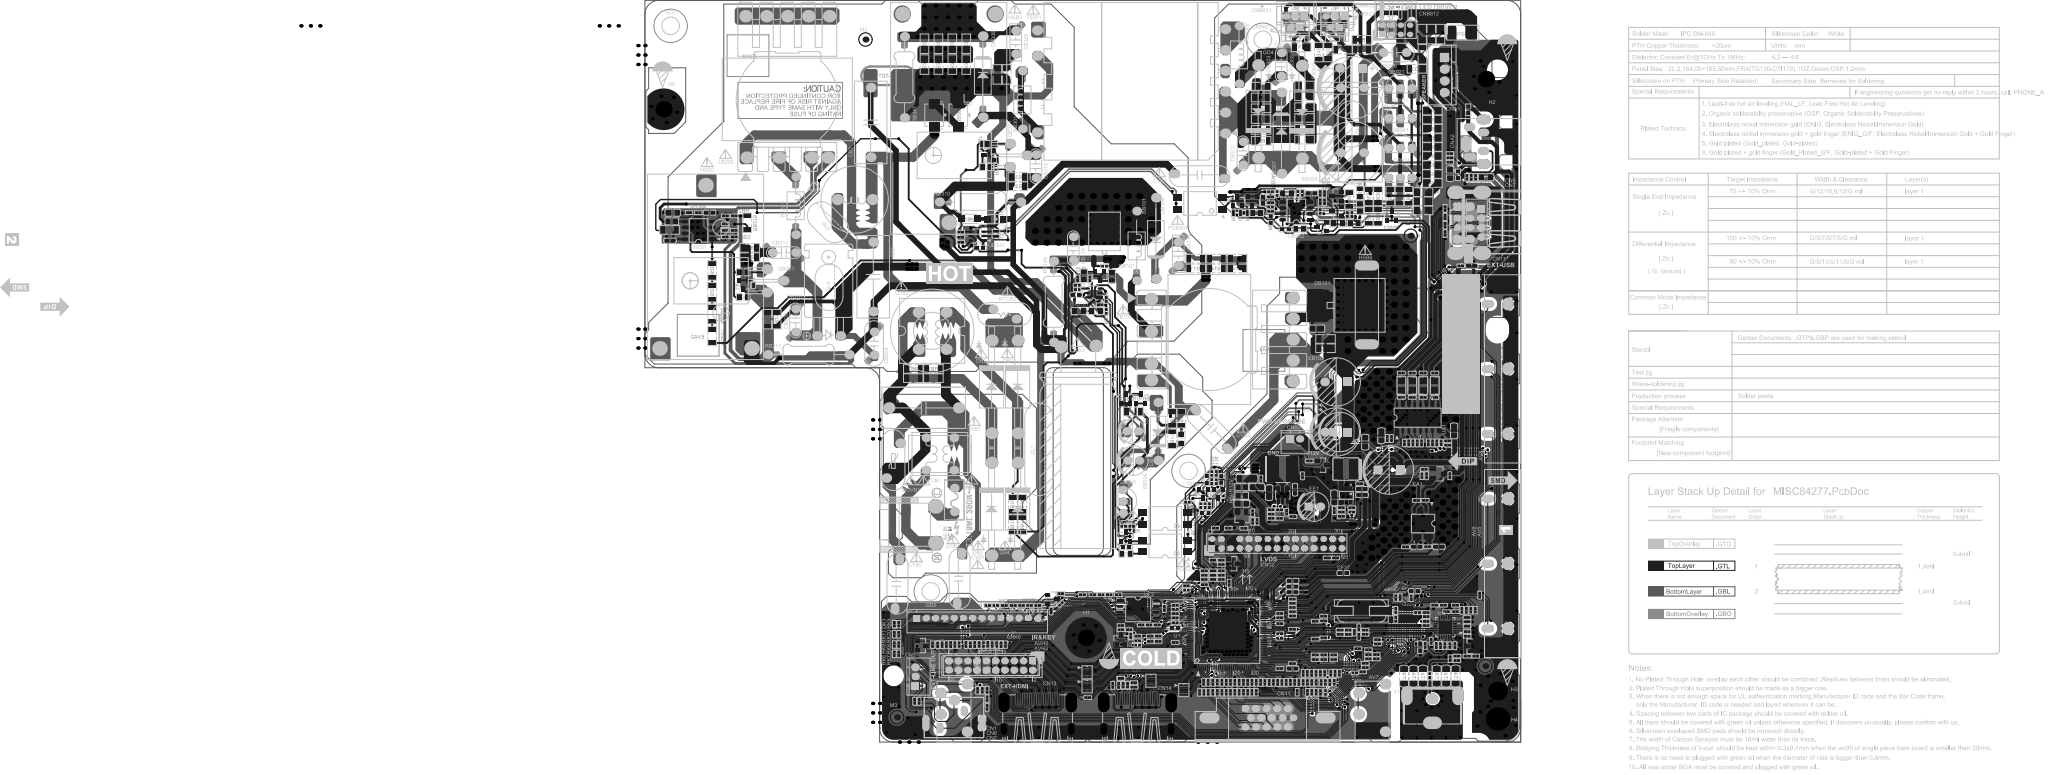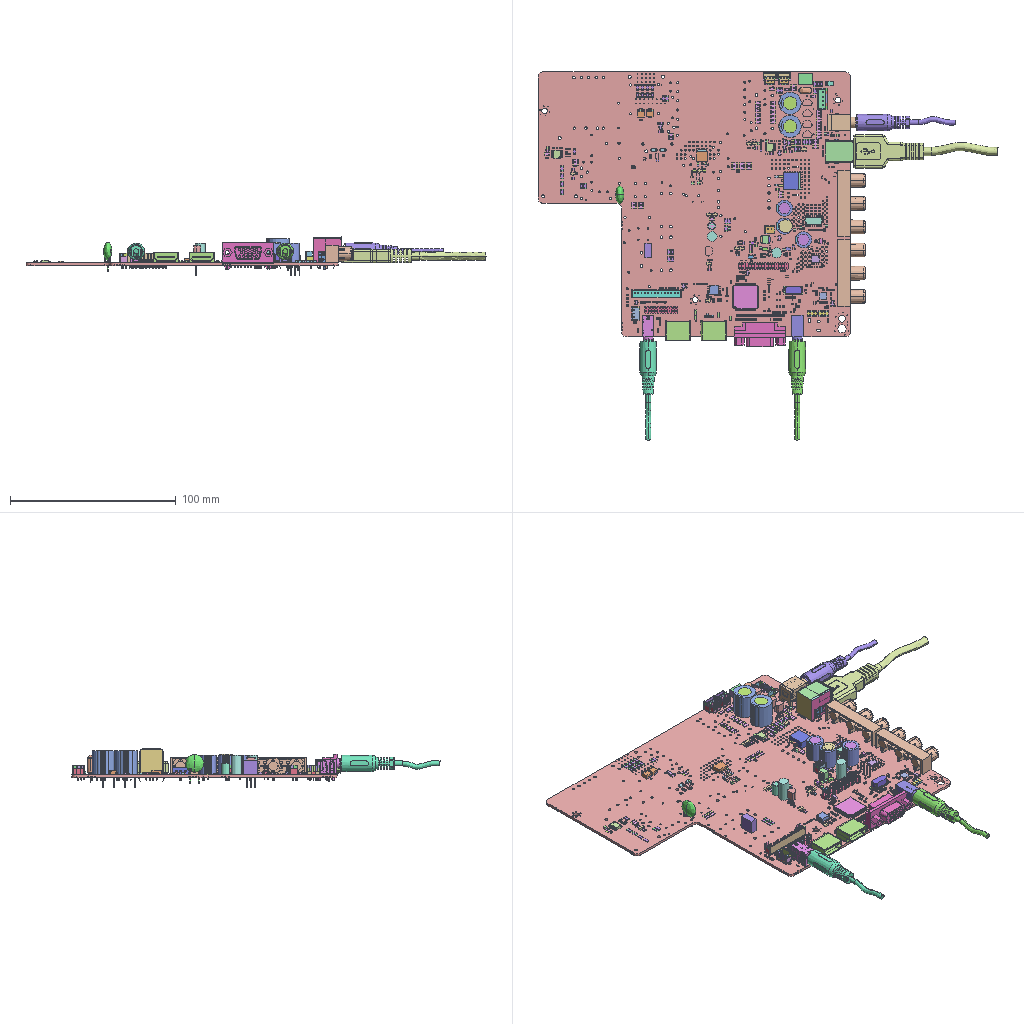Circuit board layout | Altium Designer | box 277.7 x 222.2 x 23.8 mm
Layer stack:
# Altium Designer layer stack of  (unit mm; dielectric type: 0 none, 1 core, 2 prepreg, 3 surface material)
index,name,kind,layer,copper_thickness_mm,dielectric_type,dielectric_thickness_mm,dielectric_material,dielectric_constant
0,TopPaste,other,,,,,,
1,TopOverlay,other,,,,,,
2,TopSolder,dielectric,,,3,0.0102,Solder Resist,3.5
3,TopLayer,copper,TopLayer,0.0356,,,,
4,Dielectric1,dielectric,,,1,1.5,FR-4,4.8
5,BottomLayer,copper,BottomLayer,0.0356,,,,
6,BottomSolder,dielectric,,,3,0.0102,Solder Resist,3.5
7,BottomOverlay,other,,,,,,
8,BottomPaste,other,,,,,,
# drill layer pairs: low layer,high layer
drill_pair,TopLayer,BottomLayer
Part placement, first 448 of 710 lines:
Designator,Comment,Layer,Footprint,Center-X(mm),Center-Y(mm),Rotation
NO DOLBY,NO DOLBY,BottomLayer,NO_DOLBY-SILK,-669.474,-465.296,360
CNB1,Connect jack, 2Pin, D7.92, L, SNAP, Fool-proofing, nature, L=2.8mm, DIP, AMA,TopLayer,CON2-H7.92,-126,46.889,360
S/N1,Barcode,TopLayer,Barcode,-669.474,-465.296,90
EVA6,NC/7×7×3mm-C-4305 fireproof foam-black,BottomLayer,EVA(7*7*3),-669.474,-465.296,180
S/N2,Barcode,BottomLayer,BARCODE,-669.474,-465.296,0
UF2,SPI FLASH chip, IC SPI FLASH, 32Mb, SOIC8, SMD, GD25Q32CSIG, GigaDevice,TopLayer,SOIC8,-82.347,28.626,360
RH20,NC/NC/100ohm-0402-±5%-1/16W,TopLayer,R0402,-86.063,24.232,180
RH19,NC/NC/100ohm-0402-±5%-1/16W,TopLayer,R0402,-86.063,25.138,180
AVH3,NC/gold pin, pin connector, 2×10Pin, D, D2.0mm, L=2.6mm, DIP, LK,TopLayer,SIP2*10/2.0DM-1,-114.1,16.518,360
AVH2,NC/NC/connect jack, 2×10Pin, D2.0, D, SNAP, Fool-proofing, Beige, L=2.6mm, DIP, CJ,TopLayer,SIP2*10/2.0D-4,-114.1,16.518,360
RT7,FCM1005KF-121T06(120ohm-500mA),TopLayer,R0402,-23.581,31.1,270
RT12,430ohm-0402-±5%-1/16W,TopLayer,R0402,-35.8,23.7,90
LF7,0ohm-0402-±5%-1/16W,TopLayer,L0402,-20.371,27.058,0
CT2,NC/10uF-0603-X5R-±20%-6.3V,TopLayer,C0603,-22.835,32.558,360
CF39,NC/4.7pF-0402-NPO-±5%-50V,TopLayer,C0402,-20.371,27.94,180
CF33,1000pF-0402-X7R-±10%-50V,TopLayer,C0402,-22.2,27.94,180
CF32,1Kohm-0402-±5%-1/16W,TopLayer,C0402,-26.9,28.407,90
UB102,AZ431AN-ATRE1(BCD),TopLayer,SOT-23-RAK,-65.15,53.575,180
RB135,18Kohm-0402-±1%-1/16W,TopLayer,R0402,-65.55,56.15,90
RB134,4K7ohm-0402-±1%-1/16W,TopLayer,R0402,-65.55,57.95,90
RB133,3Kohm-0402-±1%-1/16W,TopLayer,R0402,-66.5,57.95,270
RB132,3Kohm-0402-±1%-1/16W,TopLayer,R0402,-71.75,51.75,180
RB131,2Kohm-0603-±5%-1/10W,TopLayer,R0603,-64.45,56.65,90
CB110,NC/1000pF-0402-X7R-±10%-50V,TopLayer,C0402,-66.5,56.15,90
CB109,0.1uF-0603-X7R-±10%-50V,TopLayer,C0603,-67.6,56.65,90
RB386,9K1ohm-0402-±1%-1/16W,TopLayer,R0402,-68.879,50.952,270
RB385,4K7ohm-0402-±1%-1/16W,TopLayer,R0402,-67.952,50.952,90
RB384,1Kohm-0603-±1%-1/10W,TopLayer,R0603,-67.952,49.4,180
QB305,LMBT3904LT1G,TopLayer,SOT-23,-68.35,53.575,360
CB327,0.1uF-0402-X7R-±10%-16V,TopLayer,C0402,-67.029,50.952,270
RB146,100Kohm-1206-±5%-1/4W,TopLayer,R1206,-65.515,102.159,360
RB145,100Kohm-1206-±5%-1/4W,TopLayer,R1206,-61.068,104.286,360
RB144,100Kohm-1206-±5%-1/4W,TopLayer,R1206,-65.515,104.286,360
HSB2,40×25×5.0-black-with pins (thickness=1.5mm)-FR,TopLayer,HS018,-175.489,102.514,0
DB105,FR107 (tape and reel/LRC),TopLayer,D1-H-12.5,-78.08,67.018,270
DB202,NC/GS3J-B(GULF),TopLayer,DIODE-SMB-1,-126.287,135.215,270
DB370,NC/FF7,TopLayer,DIODE-S-14,-118.624,112.856,180
DB371,NC/FF7,TopLayer,DIODE-S-14,-113.05,112.827,180
GL3,NC/SLD-8854W,TopLayer,Silica_gel-10,-669.474,-465.296,45
RB347,NC/MOF-300Kohm-±5%-2WS (tape and reel/Futaba),TopLayer,R2-H-17.5,-132.664,143.421,270
LF5,NC,TopLayer,GND,-73.937,26.294,270
LF3,NC,TopLayer,GND,-49.345,22.913,360
LF2,NC,TopLayer,GND,-52.903,16.325,135
LF1,NC,TopLayer,GND,-49.373,23.531,360
C1,NC/10uF-1206-X5R-±10%-16V,TopLayer,C1206,-58.95,56.85,360
H5,Location hole,TopLayer,ASSE3.5C-3,-184.446,136.466,0
M3,MARK,TopLayer,MARK,-134.254,5.359,0
M2,MARK,TopLayer,MARK,-141.05,151.55,0
COLD,COLD,TopLayer,COLD,-669.474,-465.296,360
CAUTION,CAUTION,BottomLayer,CAUTION,-669.474,-465.296,180
T1,RF connector,RF JACK,H,IEC,T14.5,CH6.3,12.4×13.2×7.7mm,DIP,LHD-020 assembly,LHD,TopLayer,ANT-IEC14.5-H-短体-NG,-19,7.079,360
CD5,10uF-0805-X5R-±20%-16V,TopLayer,C0805,-54.171,53.831,270
5V_STB,TEST,BottomLayer,TP,-33.96,47.024,90
CM2,0.1uF-0402-X5R-±20%-16V,TopLayer,C0402,-15.265,57.455,270
QM1,WPM2341A-3/TR,TopLayer,SOT-23-1,-17.78,57.861,90
??,NC/glue, 0.1g, silicone,TopLayer,HEAT-SHRINKABLE_TUBE,-1.778,1.778,90
CN17,NC/4PIN-2.0-D-H-G,TopLayer,SIP4/2.0D-1,-8.521,111.989,270
RA14,NC/120ohm-0402-±5%-1/16W,TopLayer,R0402,-15.246,126.944,360
RA17,NC/0ohm-0603-±5%-1/10W,TopLayer,R0603,-11.3,136.4,90
RA9,NC/120ohm-0402-±5%-1/16W,TopLayer,R0402,-11.59,121.831,90
CA41,10uF-0805-X5R-±20%-16V,TopLayer,C0805,-15.197,122.616,270
CA40,10uF-0805-X5R-±20%-16V,TopLayer,C0805,-7.475,121.831,360
CA61,6800pF-0402-X7R-±10%-50V,TopLayer,C0402,-15.246,126.022,180
CA60,6800pF-0402-X7R-±10%-50V,TopLayer,C0402,-10.663,121.831,270
RA10,NC/0ohm-0603-±5%-1/10W,TopLayer,R0603,-13.503,122.372,90
RA23,1Kohm-0402-±5%-1/16W,TopLayer,R0402,-9.723,121.831,270
RA28,1Kohm-0402-±5%-1/16W,TopLayer,R0402,-15.246,125.092,180
U1,TV main chip,IC Main Chip,TSUMV56RUU-Z1,32bit,Single-Core,QFP,SMD,Mstar,TopLayer,QFP128/0.4-5,-63.232,24.046,0
M1,MARK,TopLayer,MARK,-7.62,16.383,0
H4,Location hole,TopLayer,ASSE5.0C-4,-5.267,5.093,0
H3,Location hole,TopLayer,ASSE4.0C-4,-5.216,11.22,0
H2,Location hole,TopLayer,ASSE3.5C-3,-7.436,143.528,0
H1,Location hole,TopLayer,ASSE3.5C-3,-93.537,22.466,0
CNA2,PJ-339,TopLayer,PHONE-HD-12,-7.45,129.5,90
CNA1,Connect jack, 4Pin, D2.50, D, L=2.8mm, DIP, LD,TopLayer,SIP4/2.54D-1,-16.421,143.887,270
CN14,161011041,TopLayer,HDMI-HS-1,-82.5,5.92,0
CN13,161011041,TopLayer,HDMI-HS-1,-104,5.92,0
CN11,WLHD-051A,TopLayer,DB15-HF-1,-54.5,5.251,0
CN7,NC/USB-042M-002DP,TopLayer,USB1-HD-2,-9.655,112,90
CN6,NC/earphone terminal, Earphone Jack, H, F3.5, CH7.0, Black, switch, Seal, DIP, PJ7724-F05L3BY-D, YUQIU,TopLayer,PHONE-HD-42,-122.1,7.371,0
CN5,WLUS-074B,TopLayer,USB2-HD-1,-11.15,112,90
CN2,NC/RCA terminal, RCA Jack, AV1, H, Orange, CH5.5, Seal, DIP, AV38A-01S-5020, QS,TopLayer,AV1-H-4,-122.002,6.546,0
CN1,RCA terminal, RCA Jack, AV1, H, Yellow, CH5.5, Seal, DIP, AV38A-01S-5030, QS,TopLayer,AV1-H-4,-122.002,6.546,0
AV8,RCA terminal, RCA Jack, AV3, H, Yellow, White, Red, CH5.5, D14, Seal, DIP, RC075-F03L3BY-A, YUQIU (MI material),TopLayer,AV3-H14-15,-4.925,80.5,90
AV7,Earphone terminal, Earphone Jack, H, F3.5, CH7.0, Black, Seal, DIP, PJ7723-F03L3BY-C, YUQIU,TopLayer,PHONE-HD-41,-32.05,7.375,0
AV5,NC/RCA terminal, RCA Jack, AV3, H, Green, Blue, Red, CH5.5, D14, Seal, DIP, RC075-F03L3BY-B, YUQIU (MI material),TopLayer,AV3-H14-15,-4.925,38.5,90
AV2,RCA terminal, RCA Jack, AV3, H, Yellow, White, Red, CH5.5, D14, Seal, DIP, RC075-F03L3BY-A, YUQIU (MI material),TopLayer,AV3-H14-15,-4.925,38.5,90
CQC,CQC,TopLayer,CQC,-669.474,-465.296,270
Manufacture_Info,Manufacture_Info,TopLayer,MANUFACTURE_INFO,-36.802,95.208,360
XXXXXXXXXXXX,PCB_NAME,TopLayer,PCB_NAME,-39.624,32.334,90
CA23,0.1uF-0402-X5R-±20%-16V,TopLayer,C0402,-28.727,65.481,90
RA8,4K7ohm-0402-±5%-1/16W,TopLayer,R0402,-64.44,38.303,180
CA22,0.22uF-0402-X5R-±10%-16V,TopLayer,C0402,-18.491,74.346,180
CA13,0.22uF-0402-X5R-±10%-16V,TopLayer,C0402,-21.006,74.346,360
CA12,0.22uF-0402-X5R-±10%-16V,TopLayer,C0402,-23.368,74.346,180
CA20,0.22uF-0402-X5R-±10%-16V,TopLayer,C0402,-18.986,64.529,270
CA21,0.22uF-0402-X5R-±10%-16V,TopLayer,C0402,-19.907,64.529,270
CA15,1uF-0402-X5R-±20%-16V,TopLayer,C0402,-21.361,64.529,90
RA1,4K7ohm-0402-±5%-1/16W,TopLayer,R0402,-64.44,36.932,360
CA9,1000pF-0402-X7R-±10%-50V,TopLayer,C0402,-15.723,64.058,180
CA10,2200pF-0402-X7R-±10%-50V,TopLayer,C0402,-18.491,79.604,360
CA11,0.1uF-0402-X5R-±20%-16V,TopLayer,C0402,-15.723,64.973,180
CA14,0.22uF-0402-X5R-±10%-16V,TopLayer,C0402,-25.705,74.346,360
CA17,2200pF-0402-X7R-±10%-50V,TopLayer,C0402,-21.006,79.604,180
LBA1,UPZ2012E601-2R0TF(600ohm-2000mA),TopLayer,L0805,-25.705,76.911,90
LBA2,UPZ2012E601-2R0TF(600ohm-2000mA),TopLayer,L0805,-23.368,76.911,90
LBA3,UPZ2012E601-2R0TF(600ohm-2000mA),TopLayer,L0805,-21.006,76.911,90
LBA4,UPZ2012E601-2R0TF(600ohm-2000mA),TopLayer,L0805,-18.491,76.911,90
CT46,NC/4700pF-1206-X7R-±10%-1000V,TopLayer,C1206,-14.026,14.243,270
CT43,0ohm-1206-±5%-1/4W,TopLayer,C1206,-18.09,14.243,270
CT42,0ohm-1206-±5%-1/4W,TopLayer,C1206,-16.058,14.243,270
CT41,0ohm-1206-±5%-1/4W,TopLayer,C1206,-21.049,14.218,270
CT44,0ohm-1206-±5%-1/4W,TopLayer,C1206,-23.081,14.218,270
CT40,470pF-0402-X7R-±10%-50V,TopLayer,C0402,-19.563,14.307,90
CT45,NC/4700pF-1206-X7R-±10%-1000V,TopLayer,C1206,-25.113,14.218,270
RT4,4K7ohm-0402-±5%-1/16W,TopLayer,R0402,-25.951,31.168,270
RT3,4K7ohm-0402-±5%-1/16W,TopLayer,R0402,-26.9,31.168,270
CT30,0.1uF-0402-X5R-±20%-16V,TopLayer,C0402,-18.517,29.54,360
CT9,0.1uF-0402-X5R-±20%-16V,TopLayer,C0402,-14.161,20.813,270
CT11,0.022uF-0402-X7R-±10%-16V,TopLayer,C0402,-17.271,20.837,90
CT12,0.022uF-0402-X7R-±10%-16V,TopLayer,C0402,-18.186,20.837,270
CT18,0.1uF-0402-X5R-±20%-16V,TopLayer,C0402,-19.281,21.742,90
CT21,0.047uF-0402-X7R-±10%-16V,TopLayer,C0402,-11.573,25.969,360
CT25,0.1uF-0402-X5R-±20%-16V,TopLayer,C0402,-12.673,28.414,90
CT26,330pF-0402-NPO-±5%-50V,TopLayer,C0402,-16,28.135,360
CT27,0.1uF-0402-X5R-±20%-16V,TopLayer,C0402,-16.647,29.527,360
CT29,6800pF-0402-X7R-±10%-50V,TopLayer,C0402,-14.044,29.527,360
DT1,BAV99-BR,TopLayer,SO-23,-10.671,20.686,270
LT1,SDCL1005C68NJTDF(68nH-0402±5%-C),TopLayer,L0402,-15.244,20.813,90
LT2,GZ1005U102CTF(1000ohm-300mA),TopLayer,L0402,-16.326,20.813,270
LT6,GZ1005U102CTF(1000ohm-300mA),TopLayer,L0402,-11.534,22.846,360
LT8,GZ1005U102CTF(1000ohm-300mA),TopLayer,L0402,-11.55,23.81,360
LT10,SDCL1005CR18JTDF(180nH-0402±5%-C),TopLayer,L0402,-11.569,25.028,360
RT11,1K8ohm-0402-±5%-1/16W,TopLayer,R0402,-14.044,28.135,180
CT7,30pF-0402-NPO-±5%-50V,TopLayer,C0402,-11.709,28.444,270
CT8,30pF-0402-NPO-±5%-50V,TopLayer,C0402,-11.573,26.884,180
RT5,33ohm-0402-±5%-1/16W,TopLayer,R0402,-10.743,28.444,270
RT6,33ohm-0402-±5%-1/16W,TopLayer,R0402,-9.795,28.459,270
UT1,Silicon tuner, IC Si Tuner, QFN24, SMD, R842, Rafael,TopLayer,QFN24/0.5-3,-16.254,24.773,180
CA16,2200pF-0402-X7R-±10%-50V,TopLayer,C0402,-23.368,79.604,180
CA18,0.22uF-0402-X5R-±10%-16V,TopLayer,C0402,-23.202,64.529,270
CA19,0.22uF-0402-X5R-±10%-16V,TopLayer,C0402,-22.282,64.529,270
CA24,1000pF-0402-X7R-±10%-50V,TopLayer,C0402,-27.813,65.481,90
CA25,2200pF-0402-X7R-±10%-50V,TopLayer,C0402,-25.705,79.604,180
CA31,3300pF-0402-X7R-±10%-50V,TopLayer,C0402,-24.123,64.529,90
CA32,3300pF-0402-X7R-±10%-50V,TopLayer,C0402,-18.065,64.529,270
CD1,10uF-0805-X5R-±20%-16V,TopLayer,C0805,-56.799,54.974,180
CD2,1uF-0402-X5R-±20%-6.3V,TopLayer,C0402,-49.035,48.652,180
CD3,0.1uF-0402-X5R-±20%-16V,TopLayer,C0402,-46.987,57.44,90
CD4,10uF-0603-X5R-±20%-6.3V,TopLayer,C0603,-48.587,54.44,90
CD6,0.1uF-0402-X5R-±20%-16V,TopLayer,C0402,-55.936,56.734,90
CD7,8pF-0402-NPO-±5%-50V,TopLayer,C0402,-51.918,50.089,360
CD8,NC/10uF-0805-X5R-±20%-16V,TopLayer,C0805,-29.997,66.091,90
CD11,10uF-0805-X5R-±20%-16V,TopLayer,C0805,-40.132,52.68,270
CD12,0.1uF-0402-X5R-±20%-16V,TopLayer,C0402,-40.132,49.936,270
CD13,NC/NC/3300pF-0402-X7R-±10%-50V,TopLayer,C0402,-38.608,48.692,360
CD14,10uF-0603-X5R-±20%-6.3V,TopLayer,C0603,-34.214,54.585,360
CD15,10uF-0603-X5R-±20%-6.3V,TopLayer,C0603,-34.163,53.315,360
CD16,0.1uF-0402-X5R-±20%-16V,TopLayer,C0402,-34.646,55.728,360
CD17,1uF-0402-X5R-±20%-6.3V,TopLayer,C0402,-36.347,50.546,360
CF2,0.1uF-0402-X5R-±20%-16V,TopLayer,C0402,-76.708,28.829,90
CF6,0.1uF-0402-X5R-±20%-16V,TopLayer,C0402,-62.763,34.29,270
CF8,0.1uF-0402-X5R-±20%-16V,TopLayer,C0402,-74.397,27.711,360
CF16,1uF-0402-X5R-±20%-6.3V,TopLayer,C0402,-74.397,29.489,360
CF17,1uF-0402-X5R-±20%-6.3V,TopLayer,C0402,-68.123,33.96,360
CF21,1uF-0402-X5R-±20%-6.3V,TopLayer,C0402,-74.397,28.626,360
CF23,1uF-0402-X5R-±20%-6.3V,TopLayer,C0402,-74.397,25.705,360
CF25,1uF-0402-X5R-±20%-6.3V,TopLayer,C0402,-74.397,26.797,360
CF35,NC/5pF-0402-NPO-±5%-50V,TopLayer,C0402,-39.846,39.721,180
CF36,NC/5pF-0402-NPO-±5%-50V,TopLayer,C0402,-41.646,39.721,180
CF37,NC/10uF-0603-X5R-±20%-6.3V,TopLayer,C0603,-38.202,36.474,360
CG1,NC/0.1uF-0402-X5R-±20%-16V,TopLayer,C0402,-68.123,36.932,360
CH3,NC/0.1uF-0402-X5R-±20%-16V,TopLayer,C0402,-119.423,21.036,270
CH4,NC/0.1uF-0402-X5R-±20%-16V,TopLayer,C0402,-122.725,21.034,270
CH7,NC/30pF-0402-NPO-±5%-50V,TopLayer,C0402,-83.259,11.847,180
CH8,NC/0.1uF-0402-X5R-±20%-16V,TopLayer,C0402,-87.833,12.243,270
CH9,NC/0.1uF-0402-X5R-±20%-16V,TopLayer,C0402,-86.563,12.243,90
CH10,NC/30pF-0402-NPO-±5%-50V,TopLayer,C0402,-93.21,9.604,180
CI8,NC/100pF-0402-NPO-±5%-50V,TopLayer,C0402,-8.839,31.699,90
CK1,NC/0.1uF-0402-X5R-±20%-16V,TopLayer,C0402,-101.107,28.275,90
CK2,0.01uF-0402-X7R-±10%-50V,TopLayer,C0402,-94.361,31.775,180
CK3,NC/0.1uF-0402-X5R-±20%-16V,TopLayer,C0402,-103.927,29.464,360
CK6,NC/10pF-0402-NPO-±5%-50V,TopLayer,C0402,-111.173,29.464,180
CK10,NC/0.1uF-0402-X5R-±20%-16V,TopLayer,C0402,-109.251,29.464,360
CL2,0.1uF-0402-X5R-±20%-16V,TopLayer,C0402,-22.454,52.121,360
CL3,0.1uF-0402-X5R-±20%-16V,TopLayer,C0402,-24.8,42.102,180
CL4,NC/10uF-0603-X5R-±20%-6.3V,TopLayer,C0603,-22.377,42.139,360
CL42,0.1uF-0402-X5R-±20%-16V,TopLayer,C0402,-20.574,52.146,360
CL43,0.1uF-0402-X5R-±20%-16V,TopLayer,C0402,-20.034,42.139,360
CL44,10uF-0603-X5R-±20%-6.3V,TopLayer,C0603,-17.628,42.139,360
CM1,0.22uF-0402-X5R-±10%-16V,TopLayer,C0402,-20.269,57.455,90
CM3,NC/0.1uF-0402-X5R-±20%-16V,TopLayer,C0402,-57.709,49.454,90
CM4,0.1uF-0402-X5R-±20%-16V,TopLayer,C0402,-65.71,46.152,180
CM5,NC/10uF-0805-X5R-±20%-16V,TopLayer,C0805,-60.046,51.435,180
CM7,0.022uF-0402-X7R-±10%-16V,TopLayer,C0402,-59.588,46.126,360
CO6,NC/0.1uF-0402-X5R-±20%-16V,TopLayer,C0402,-130.472,8.809,90
CO7,NC/330pF-0402-NPO-±5%-50V,TopLayer,C0402,-129.504,8.809,90
CO8,NC/NC/10pF-0402-NPO-±5%-50V,TopLayer,C0402,-78.257,25.258,360
CO10,NC/NC/4700pF-0402-X7R-±10%-50V,TopLayer,C0402,-114.882,11.168,90
CO11,NC/NC/4700pF-0402-X7R-±10%-50V,TopLayer,C0402,-114.882,7.516,90
CT13,NC/1.2pF-0402-NPO-±0.25pf-50V,TopLayer,C0402,-13.735,18.549,360
CT17,NC/100pF-0402-NPO-±5%-50V,TopLayer,C0402,-11.534,18.549,180
CU1,10uF-0603-X5R-±20%-6.3V,TopLayer,C0603,-10.516,102.756,180
DH3,NC/NC/AVLC18S02003,TopLayer,DIODE-S0402,-116.596,21.021,90
DH4,NC/NC/AVLC18S02003,TopLayer,DIODE-S0402,-111.879,20.983,90
DH5,NC/NC/AVLC18S02003,TopLayer,DIODE-S0402,-114.722,21.044,90
DH6,NC/NC/AVLC18S02003,TopLayer,DIODE-S0402,-84.633,12.243,90
DH7,NC/NC/AVLC18S02003,TopLayer,DIODE-S0402,-85.598,12.243,90
DK1,NC/AVLC18S02003,TopLayer,DIODE-S0402,-134.848,25.391,90
EE1,470uF-10V-±20%-6.3×11-105℃-black base white print-tape and reel-F=2.5-XF,TopLayer,EC(6.3*11)-V-2.5,-44.437,50.07,180
F2,0ohm-0402-±5%-1/16W,TopLayer,R0402,-12.903,102.718,360
LD2,SCD43TL-6R8M,TopLayer,L(4.5*3.5)-S,-37.643,58.903,360
LD12,Power inductor, Power Inductor, 4.7uH, ±20%, 2.8A, 0.35×1P, DR5.8×4.5, SMD, CD54-4.7uH, wenshan,TopLayer,L(5.8*4.5)-S,-51.275,58.886,180
LT3,0ohm-0402-±5%-1/16W,TopLayer,L0402,-13.735,17.583,360
LT9,NC/SDCL1005CR27JTDF (Sunlord),TopLayer,L0402,-9.703,18.549,180
LT11,NC/SDCL1005CR27JTDF (Sunlord),TopLayer,L0402,-15.189,18,90
QH1,LMBT3904LT1G,TopLayer,SOT-23,-128.963,20.83,90
QH2,LMBT3904LT1G,TopLayer,SOT-23,-86.048,22.096,180
QK2,LMBT3904LT1G,TopLayer,SOT-23,-100.797,30.843,90
QM2,LMBT3904LT1G,TopLayer,SOT-23,-42.799,59.741,90
QM5,ME2325-G,TopLayer,SOT-23-1,-59.995,48.412,360
QM6,LMBT3904LT1G,TopLayer,SOT-23,-61.95,38.481,90
R5V,NC/0ohm-0805-±5%-1/8W,TopLayer,R0805,-60.071,53.162,180
R12V,0ohm-0805-±5%-1/8W,TopLayer,R0805,-60.063,54.974,180
RA4,1Kohm-0402-±5%-1/16W,TopLayer,R0402,-25.044,64.529,90
RA12,1Kohm-0402-±5%-1/16W,TopLayer,R0402,-17.145,64.529,90
RD1,100Kohm-0402-±1%-1/16W,TopLayer,R0402,-53.721,50.114,360
RD6,12K4ohm-0402-±1%-1/16W,TopLayer,R0402,-38.608,49.632,180
RD7,13Kohm-0402-±1%-1/16W,TopLayer,R0402,-38.608,50.571,360
RD8,68Kohm-0402-±1%-1/16W,TopLayer,R0402,-36.347,49.632,360
RD12,18Kohm-0402-±1%-1/16W,TopLayer,R0402,-51.918,48.26,360
RD13,100Kohm-0402-±1%-1/16W,TopLayer,R0402,-53.721,49.174,360
RD15,22ohm-0402-±5%-1/16W,TopLayer,R0402,-50.4,49.6,270
RD16,3K3ohm-0402-±1%-1/16W,TopLayer,R0402,-53.721,48.26,360
RF2,10Kohm-0402-±5%-1/16W,TopLayer,R0402,-88.621,31.775,180
RF3,4K7ohm-0402-±5%-1/16W,TopLayer,R0402,-86.639,31.775,180
RF8,4K7ohm-0402-±5%-1/16W,TopLayer,R0402,-71.958,32.791,180
RF9,4K7ohm-0402-±5%-1/16W,TopLayer,R0402,-71.958,33.706,180
RF13,4K7ohm-0402-±5%-1/16W,TopLayer,R0402,-66.243,35.077,180
RF18,4K7ohm-0402-±5%-1/16W,TopLayer,R0402,-68.123,35.077,180
RG1,510ohm-0402-±5%-1/16W,TopLayer,R0402,-68.123,35.992,360
RH1,10Kohm-0402-±5%-1/16W,TopLayer,R0402,-113.79,21.036,90
RH2,10Kohm-0402-±5%-1/16W,TopLayer,R0402,-112.822,21.036,90
RH3,22ohm-0402-±5%-1/16W,TopLayer,R0402,-110.927,21.036,90
RH4,22ohm-0402-±5%-1/16W,TopLayer,R0402,-115.656,21.036,90
RH5,1Kohm-0402-±5%-1/16W,TopLayer,R0402,-123.645,21.016,270
RH6,10Kohm-0402-±5%-1/16W,TopLayer,R0402,-124.562,21.003,90
RH7,10Kohm-0402-±5%-1/16W,TopLayer,R0402,-126.621,21.003,90
RH8,10Kohm-0402-±5%-1/16W,TopLayer,R0402,-79.748,22.858,360
RH9,10Kohm-0402-±5%-1/16W,TopLayer,R0402,-82.456,22.858,180
RH10,22ohm-0402-±5%-1/16W,TopLayer,R0402,-78.039,21.72,180
RH11,22ohm-0402-±5%-1/16W,TopLayer,R0402,-78.039,22.858,180
RH13,220ohm-0402-±5%-1/16W,TopLayer,R0402,-79.748,21.72,180
RH14,1Kohm-0402-±5%-1/16W,TopLayer,R0402,-84.32,24.226,360
RH15,10Kohm-0402-±5%-1/16W,TopLayer,R0402,-82.456,20.904,360
RH16,10Kohm-0402-±5%-1/16W,TopLayer,R0402,-82.456,21.844,360
RI8,10Kohm-0402-±5%-1/16W,TopLayer,R0402,-31.09,18.872,360
RI9,12Kohm-0402-±5%-1/16W,TopLayer,R0402,-32.791,18.872,360
RI10,10Kohm-0402-±5%-1/16W,TopLayer,R0402,-31.09,17.958,360
RI11,12Kohm-0402-±5%-1/16W,TopLayer,R0402,-32.791,17.958,180
RK1,22ohm-0402-±5%-1/16W,TopLayer,R0402,-98.986,29.808,225
RK2,1Kohm-0402-±5%-1/16W,TopLayer,R0402,-98.996,32.032,360
RK3,1Kohm-0402-±5%-1/16W,TopLayer,R0402,-92.1,31.775,360
RK4,4K7ohm-0402-±1%-1/16W,TopLayer,R0402,-90.348,31.775,360
RK5,510ohm-0402-±1%-1/16W,TopLayer,R0402,-133.895,25.434,270
RK6,680ohm-0402-±1%-1/16W,TopLayer,R0402,-134.848,19.036,90
RK7,1Kohm-0402-±1%-1/16W,TopLayer,R0402,-133.895,19.036,90
RK8,1K2ohm-0402-±1%-1/16W,TopLayer,R0402,-133.895,21.036,90
RK9,2K2ohm-0402-±1%-1/16W,TopLayer,R0402,-134.848,21.036,90
RK10,4K7ohm-0402-±1%-1/16W,TopLayer,R0402,-133.895,23.271,90
RK11,15Kohm-0402-±1%-1/16W,TopLayer,R0402,-134.848,23.271,90
RK15,4K7ohm-0402-±5%-1/16W,TopLayer,R0402,-114.709,29.464,360
RK16,1Kohm-0402-±5%-1/16W,TopLayer,R0402,-112.987,29.464,180
RK18,33Kohm-0402-±5%-1/16W,TopLayer,R0402,-64.44,35.077,360
RK20,10Kohm-0402-±5%-1/16W,TopLayer,R0402,-105.73,29.464,180
RK21,510ohm-0402-±5%-1/16W,TopLayer,R0402,-107.457,29.464,180
RM1,4K7ohm-0402-±5%-1/16W,TopLayer,R0402,-21.26,57.455,270
RM2,200Kohm-0402-±1%-1/16W,TopLayer,R0402,-20.752,58.852,360
RM3,10Kohm-0402-±5%-1/16W,TopLayer,R0402,-64.44,35.992,180
RM4,4K7ohm-0402-±5%-1/16W,TopLayer,R0402,-45.491,60.655,180
RM5,4K7ohm-0402-±5%-1/16W,TopLayer,R0402,-56.769,47.6,90
RM6,NC/4K7ohm-0402-±5%-1/16W,TopLayer,R0402,-62.941,46.152,360
RM7,47Kohm-0402-±1%-1/16W,TopLayer,R0402,-57.709,47.6,90
RM8,4K7ohm-0402-±5%-1/16W,TopLayer,R0402,-66.243,39.243,360
RM10,2K2ohm-0402-±5%-1/16W,TopLayer,R0402,-64.44,39.243,360
RO3,NC/47Kohm-0402-±5%-1/16W,TopLayer,R0402,-114.882,9.385,270
RO6,0ohm-0402-±5%-1/16W,TopLayer,R0402,-116.921,11.168,90
RO7,NC/47Kohm-0402-±5%-1/16W,TopLayer,R0402,-115.902,11.168,90
RO9,NC/220ohm-0402-±5%-1/16W,TopLayer,R0402,-80.01,25.258,180
RO10,NC/100ohm-0402-±5%-1/16W,TopLayer,R0402,-81.722,25.258,180
UD2,LC2127CB5TR,TopLayer,SOT-23-5,-37.508,53.223,180
UD11,MP1470GJ-Z,TopLayer,SOT-23-6,-51.224,53.298,180
UL1,LC1118CS8TR1833,TopLayer,SOP8/1.27-3,-21.031,47.142,270
RH55,NC/33Kohm-0402-±5%-1/16W,TopLayer,R0402,-121.806,21.034,270
RH56,NC/22Kohm-0402-±5%-1/16W,TopLayer,R0402,-120.896,21.036,270
CN3,NC/3PIN-2.0-D-H-G,TopLayer,SIP3/2.0D-1,-130.341,14.132,90
CF18,1uF-0402-X5R-±20%-6.3V,TopLayer,C0402,-74.397,21.488,360
CH15,NC/1uF-0402-X5R-±20%-6.3V,TopLayer,C0402,-117.538,21.031,270
CN12,2×15PIN-2.0-D-H-M(pin length=2.6mm)-LD(missing 6PIN),TopLayer,SIP2*15/2.0D-2,-52.516,42.81,180
UA1,Audio amplifier, IC Audio AMP, Class D, 2×13W@13V@8ohm, TSSOP-16, SMD, CSY1281AER, ON-Bright,TopLayer,SOP16/1.27-7,-22.2,69.975,90
CF3,10uF-0603-X5R-±20%-6.3V,TopLayer,C0603,-74.397,24.638,180
LF4,NC,TopLayer,GND,-73.984,29.065,90
M4,MARK,TopLayer,MARK,-23.688,109.222,0
CD9,NC/10uF-0805-X5R-±20%-16V,TopLayer,C0805,-14.351,67.132,270
CD10,10uF-0805-X5R-±20%-16V,TopLayer,C0805,-33.484,64.695,270
CG2,NC/0.1uF-0402-X5R-±20%-16V,TopLayer,C0402,-66.243,36.932,360
RG2,0ohm-0402-±5%-1/16W,TopLayer,R0402,-66.243,35.992,180
RV13,10Kohm-0402-±5%-1/16W,TopLayer,R0402,-65.329,10.744,90
RV12,100ohm-0402-±5%-1/16W,TopLayer,R0402,-66.294,10.744,90
RV11,75ohm-0402-±5%-1/16W,TopLayer,R0402,-63.398,10.744,270
RV9,33ohm-0402-±5%-1/16W,TopLayer,R0402,-64.313,10.744,270
RF11,100ohm-0402-±5%-1/16W,TopLayer,R0402,-69.139,10.719,270
RF10,100ohm-0402-±5%-1/16W,TopLayer,R0402,-65.329,12.903,270
CV9,33pF-0402-NPO-±5%-50V,TopLayer,C0402,-66.294,12.903,270
CV7,0.047uF-0402-X7R-±10%-16V,TopLayer,C0402,-64.313,12.903,270
YF1,24MHz-±20PPM-20PF-HC-49S-SMD,TopLayer,XTAL-S-1,-34.315,28.302,180
RV8,12Kohm-0402-±5%-1/16W,TopLayer,R0402,-42.418,18.796,360
RV7,10Kohm-0402-±5%-1/16W,TopLayer,R0402,-40.259,18.796,360
RV6,10Kohm-0402-±5%-1/16W,TopLayer,R0402,-40.259,17.806,360
RV4,12Kohm-0402-±5%-1/16W,TopLayer,R0402,-42.418,17.806,180
RT18,10Kohm-0402-±5%-1/16W,TopLayer,R0402,-42.418,22.479,180
RT14,0ohm-0402-±5%-1/16W,TopLayer,L0402,-37.139,23.236,180
RT10,220ohm-0402-±5%-1/16W,TopLayer,R0402,-33.501,23.261,360
RT9,220ohm-0402-±5%-1/16W,TopLayer,R0402,-33.501,24.15,360
RT1,0ohm-0402-±5%-1/16W,TopLayer,L0402,-37.139,24.163,180
RF15,200Kohm-0402-±5%-1/16W,TopLayer,R0402,-30.836,22.098,360
RF14,200Kohm-0402-±5%-1/16W,TopLayer,R0402,-32.791,19.914,360
RF1,NC/1Mohm-0402-±5%-1/16W,TopLayer,R0402,-44.247,26.081,180
RA11,NC,BottomLayer,GND,-27.153,19.355,270
RA7,NC,BottomLayer,GND,-29.159,21.119,270
CT24,33pF-0402-NPO-±5%-50V,TopLayer,C0402,-34.849,22.809,90
CT23,0.1uF-0402-X5R-±20%-16V,TopLayer,C0402,-38.887,23.236,180
CT20,0.1uF-0402-X5R-±20%-16V,TopLayer,C0402,-38.887,24.163,180
CT19,NC/0.022uF-0402-X7R-±10%-16V,TopLayer,C0402,-44.247,22.2,360
CT10,33pF-0402-NPO-±5%-50V,TopLayer,C0402,-34.847,24.633,90
CT6,10uF-0603-X5R-±20%-6.3V,TopLayer,C0603,-21.631,20.457,270
CF38,NC/NC/30pF-0402-NPO-±5%-50V,TopLayer,C0402,-26.9,26.507,90
CF30,NC/1000pF-0402-X7R-±10%-50V,TopLayer,C0402,-30.836,21.184,180
CF29,NC/1000pF-0402-X7R-±10%-50V,TopLayer,C0402,-35.052,20.142,180
CF24,1uF-0402-X5R-±20%-6.3V,TopLayer,C0402,-51.86,26.822,180
CF20,1uF-0402-X5R-±20%-6.3V,TopLayer,C0402,-51.86,25.552,180
CF19,1uF-0402-X5R-±20%-6.3V,TopLayer,C0402,-51.867,27.737,180
CF14,0.1uF-0402-X5R-±20%-16V,TopLayer,C0402,-51.86,22.377,180
CF12,0.1uF-0402-X5R-±20%-16V,TopLayer,C0402,-51.86,23.393,180
CF10,0.1uF-0402-X5R-±20%-16V,TopLayer,C0402,-49.149,27.203,180
CF9,0.1uF-0402-X5R-±20%-16V,TopLayer,C0402,-49.149,24.333,360
CF4,30pF-0402-NPO-±5%-50V,TopLayer,C0402,-42.418,26.136,180
CF1,30pF-0402-NPO-±5%-50V,TopLayer,C0402,-42.418,27.153,180
CT5,0.1uF-0402-X5R-±20%-16V,TopLayer,C0402,-20.568,20.853,90
CT1,0.1uF-0402-X5R-±20%-16V,TopLayer,C0402,-20.374,25.131,360
RT2,100ohm-0402-±5%-1/16W,TopLayer,R0402,-20.38,26.046,360
HS,NC/14×14×06-THD,TopLayer,HS-S,-669.474,-465.296,0
DU1,NC/AIES12U020R2,TopLayer,DIODE-S0402,-45.923,10.744,270
CF7,0.1uF-0402-X5R-±20%-16V,TopLayer,C0402,-59.69,12.903,90
CF13,0.1uF-0402-X5R-±20%-16V,TopLayer,C0402,-51.86,15.875,180
CF26,0.047uF-0402-X7R-±10%-16V,TopLayer,C0402,-49.581,12.878,270
CF27,0.1uF-0402-X5R-±20%-16V,TopLayer,C0402,-49.149,16.937,180
CF28,10uF-0603-X5R-±20%-6.3V,TopLayer,C0603,-49.124,15.87,360
CF31,0.047uF-0402-X7R-±10%-16V,TopLayer,C0402,-62.484,12.903,270
CF34,0.047uF-0402-X7R-±10%-16V,TopLayer,C0402,-56.007,12.878,270
CI1,0.047uF-0402-X7R-±10%-16V,TopLayer,C0402,-52.324,12.878,270
CI2,NC/100pF-0402-NPO-±5%-50V,TopLayer,C0402,-50.495,12.878,90
CI3,1uF-0402-X5R-±20%-6.3V,TopLayer,C0402,-46.838,14.834,270
CI4,1uF-0402-X5R-±20%-6.3V,TopLayer,C0402,-45.009,14.834,270
CI5,1uF-0402-X5R-±20%-6.3V,TopLayer,C0402,-33.477,16.993,360
CI6,1uF-0402-X5R-±20%-6.3V,TopLayer,C0402,-33.477,16.078,360
CI7,0.047uF-0402-X7R-±10%-16V,TopLayer,C0402,-57.861,12.903,270
CI9,NC/0.047uF-0402-X7R-±10%-16V,TopLayer,C0402,-58.776,12.903,270
CI11,NC/0.047uF-0402-X7R-±10%-16V,TopLayer,C0402,-54.153,12.878,270
CO1,NC/1uF-0402-X5R-±20%-6.3V,TopLayer,C0402,-39.98,14.834,90
CO4,NC/1uF-0402-X5R-±20%-6.3V,TopLayer,C0402,-41.097,12.878,90
CO9,100pF-0402-NPO-±5%-50V,TopLayer,C0402,-47.752,12.878,90
CV1,0.047uF-0402-X7R-±10%-16V,TopLayer,C0402,-60.63,12.903,270
CV3,0.047uF-0402-X7R-±10%-16V,TopLayer,C0402,-63.398,12.903,270
CV5,1uF-0402-X5R-±20%-6.3V,TopLayer,C0402,-44.247,17.805,180
CV6,1uF-0402-X5R-±20%-6.3V,TopLayer,C0402,-44.247,18.796,180
CV10,33pF-0402-NPO-±5%-50V,TopLayer,C0402,-67.285,12.903,270
LF6,NC,TopLayer,GND,-47.635,16.723,360
R3,0ohm-0402-±5%-1/16W,TopLayer,R0402,-42.037,10.7,90
R4,0ohm-0402-±5%-1/16W,TopLayer,R0402,-42.189,14.834,90
RF12,68ohm-0402-±5%-1/16W,TopLayer,R0402,-48.666,12.878,90
RF16,68ohm-0402-±5%-1/16W,TopLayer,R0402,-61.544,12.903,90
RF19,68ohm-0402-±5%-1/16W,TopLayer,R0402,-55.067,12.878,270
RI1,NC/0ohm-0402-±5%-1/16W,TopLayer,R0402,-44.044,10.744,270
RI2,0ohm-0402-±5%-1/16W,TopLayer,R0402,-44.044,12.878,270
RI3,33ohm-0402-±5%-1/16W,TopLayer,R0402,-51.41,12.878,270
RI4,10Kohm-0402-±5%-1/16W,TopLayer,R0402,-42.977,12.878,270
RI5,12Kohm-0402-±5%-1/16W,TopLayer,R0402,-45.949,14.834,270
RI6,10Kohm-0402-±5%-1/16W,TopLayer,R0402,-43.129,14.834,90
RI7,12Kohm-0402-±5%-1/16W,TopLayer,R0402,-44.069,14.834,90
RI12,33ohm-0402-±5%-1/16W,TopLayer,R0402,-56.947,12.903,90
RI13,75ohm-0402-±5%-1/16W,TopLayer,R0402,-56.947,10.744,90
RI14,NC/33ohm-0402-±5%-1/16W,TopLayer,R0402,-58.776,10.744,270
RI15,NC/75ohm-0402-±5%-1/16W,TopLayer,R0402,-57.861,10.744,270
RI16,NC/33ohm-0402-±5%-1/16W,TopLayer,R0402,-53.238,12.878,270
RI17,NC/75ohm-0402-±5%-1/16W,TopLayer,R0402,-48.133,10.744,270
RI18,75ohm-0402-±5%-1/16W,TopLayer,R0402,-43.104,10.719,90
RO1,NC/510ohm-0402-±5%-1/16W,TopLayer,R0402,-39.04,14.834,270
RO2,NC/0ohm-0402-±5%-1/16W,TopLayer,R0402,-44.983,12.878,90
RO5,NC/510ohm-0402-±5%-1/16W,TopLayer,R0402,-40.157,12.903,270
RO12,75ohm-0402-±5%-1/16W,TopLayer,R0402,-46.838,12.878,270
RO13,0ohm-0402-±5%-1/16W,TopLayer,R0402,-45.923,12.878,90
RO15,NC/0ohm-0402-±5%-1/16W,TopLayer,R0402,-42.037,12.878,90
RO16,NC/0ohm-0402-±5%-1/16W,TopLayer,R0402,-44.983,10.744,270
RO17,NC/0ohm-0402-±5%-1/16W,TopLayer,R0402,-40.894,14.834,270
RV1,33ohm-0402-±5%-1/16W,TopLayer,R0402,-60.63,10.744,270
RV2,75ohm-0402-±5%-1/16W,TopLayer,R0402,-59.69,10.744,270
RV3,33ohm-0402-±5%-1/16W,TopLayer,R0402,-62.484,10.744,270
RV5,75ohm-0402-±5%-1/16W,TopLayer,R0402,-61.544,10.744,270
RV10,100ohm-0402-±5%-1/16W,TopLayer,R0402,-67.285,10.719,90
RV14,10Kohm-0402-±5%-1/16W,TopLayer,R0402,-68.199,10.719,90
RU4,5R1ohm-0402-±5%-1/16W,TopLayer,R0402,-49.149,29.032,360
RU3,5R1ohm-0402-±5%-1/16W,TopLayer,R0402,-49.149,30.848,360
RU1,5R1ohm-0402-±5%-1/16W,TopLayer,R0402,-49.149,29.934,360
CF22,NC/10uF-0603-X5R-±20%-6.3V,TopLayer,C0603,-49.149,32.334,180
CF15,10uF-0603-X5R-±20%-6.3V,TopLayer,C0603,-49.124,34.773,180
CF5,10uF-0603-X5R-±20%-6.3V,TopLayer,C0603,-49.149,33.553,180
3V3_STB,TEST,BottomLayer,TP,-52.73,31.928,90
1.15V_STB,TEST,BottomLayer,TP,-55.499,31.496,0
RU2,5R1ohm-0402-±5%-1/16W,TopLayer,R0402,-49.149,28.118,360
DDR_1V8,TEST,BottomLayer,TP,-53.492,29.667,180
DU3,NC/AIES12U020R2,TopLayer,DIODE-S0402,-16.294,113.233,90
DU4,NC/AIES12U020R2,TopLayer,DIODE-S0402,-16.294,115.126,270
DU7,NC/AIES12U020R2,TopLayer,DIODE-S0402,-16.294,109.69,90
DU8,NC/AIES12U020R2,TopLayer,DIODE-S0402,-16.294,111.493,270
XXXXXX,PCB_TIME,TopLayer,PCB_TIME,-33.579,28.677,90
CF11,0.1uF-0402-X5R-±20%-16V,TopLayer,C0402,-68.275,12.903,90
R1,NC/0ohm-0402-±5%-1/16W,TopLayer,R0402,-34.036,15.164,180
R2,NC/0ohm-0402-±5%-1/16W,TopLayer,R0402,-35.712,14.91,180
EA1,470uF-16V±20%-10×12-105℃-tape and reel-F=5.0-XL,TopLayer,EC(10*12)-V-5,-28.308,58.703,180
RB905,NC/0ohm-1206-±5%-1/4W,TopLayer,R1206,-34.194,151.481,360
CNB2,2PIN-2.0-D-H-G-LD,TopLayer,SIP2/2.0D-1,-48.593,65.392,360
CB356,NC/CK45-B3AD102KYPNX(TDK),TopLayer,CAP8.5*4-V-5,-27.153,148.748,180
EB103,470uF-25V-±20%-10×12.5-105℃-GF-tape and reel-F=5.0 (CapXon),TopLayer,EC(10*12.5)-V-5,-39.734,77.683,180
EB102,NC/270uF-16V-±20%-8×11.5-105℃-PS-short leads-F=3.5 (Capxon),TopLayer,EC(8*11)-V-3.5,-38.959,66.888,180
EB101,470uF-25V-±20%-10×12.5-105℃-GF-tape and reel-F=5.0 (CapXon),TopLayer,EC(10*12.5)-V-5,-39.709,66.888,180
HSB6,NC/17.5×14.5×0.5- natural finish -Cu-MRD,TopLayer,HS038,-33.122,94.31,90
CNB812,NC/2×4PIN-2.0-L-H-F-gold plated-LK,TopLayer,SIP2*4H/2.0DF-1,-26.928,158.744,0
RB943,NC/10ohm-1206-±5%-1/4W,TopLayer,R1206,-19.032,120.602,180
RB942,NC/10ohm-1206-±5%-1/4W,TopLayer,R1206,-19.029,122.529,180
RB941,NC/10ohm-1206-±5%-1/4W,TopLayer,R1206,-19.032,124.463,180
RB933,NC/10ohm-1206-±5%-1/4W,TopLayer,R1206,-21.018,114.677,180
RB932,NC/10ohm-1206-±5%-1/4W,TopLayer,R1206,-21.018,116.653,180
RB931,NC/10ohm-1206-±5%-1/4W,TopLayer,R1206,-21.018,118.628,180
RB923,NC/10ohm-1206-±5%-1/4W,TopLayer,R1206,-19.032,132.316,180
RB922,NC/10ohm-1206-±5%-1/4W,TopLayer,R1206,-19.032,134.276,180
RB921,NC/10ohm-1206-±5%-1/4W,TopLayer,R1206,-19.032,136.223,180
Pad and via stacks, first 73 of 279 lines:
# Altium Designer via and pad stacks of  (unit mm). Each distinct definition once, with the count of objects using it.
# via: kind,start_layer,end_layer,hole_mm,diameter_mm,mode(0 simple;1 top-mid-bottom;2 full stack),diameter_per_layer,count,example_net
# pad: kind,layer,hole_mm,hole_type(0 round;1 square;2 slot),plating,top_size,top_shape(1 round;2 rect;3 octagon;9 rounded rect),mid_size,bottom_size,mode,footprint,size_per_layer,count,example
pad,MultiLayer,1.4,0,plated,2.2x2.2,1,2.2x2.2,2.2x2.2,0,L/LC2/15*14.5-V7.5,,2,LB1.1
pad,MultiLayer,1.4,0,plated,2x2,1,2x2,2x2,0,CAP18*8.5-V-15,,1,CXB1.2
pad,MultiLayer,1.4,0,plated,2.2x2.2,1,2.2x2.2,1.8x1.8,1,CAP18*8.5-V-15,,1,CXB1.1
pad,MultiLayer,1.2,0,plated,1.7x2.35,1,1.7x2.35,1.7x2.35,0,CAP13*4.5-V-10,,8,CYB2.2
pad,MultiLayer,0.6,2,plated,2.1x1.3,1,2.1x1.3,2.1x1.3,0,PHONE-HD-42,,1,CN6.6
pad,MultiLayer,1.4,0,plated,2.1x2.1,1,2.1x2.1,2.1x2.1,0,PHONE-HD-42,,4,CN6.3
pad,MultiLayer,0.6,2,plated,1.3x2.1,1,1.3x2.1,1.3x2.1,0,PHONE-HD-42,,1,CN6.2
pad,MultiLayer,1.4,0,plated,2.1x2.1,1,2.1x2.1,2.1x2.1,0,PHONE-HD-41,,4,AV7.1
pad,MultiLayer,1.2,2,plated,2x2.8,1,2x2.8,2x3,1,PHONE-HD-12,,2,CNA2.7
pad,MultiLayer,0.8,2,plated,1.5x2.3,1,1.5x2.3,1.5x2.3,0,PHONE-HD-12,,4,CNA2.2
pad,MultiLayer,1,2,plated,1.7x3,1,1.7x3,1.7x3,0,PHONE-HD-12,,1,CNA2.3
pad,MultiLayer,1.3,2,plated,2.6x2.3,1,2.6x2.3,2.6x2.3,0,AV3-H14-15,,9,AV2.6
pad,MultiLayer,0.8,2,plated,2.5x1.5,1,2.5x1.5,2.5x1.5,0,AV3-H14-15,,9,AV2.5
pad,MultiLayer,0.9,2,plated,1.9x1.5,1,1.9x1.5,1.9x1.5,0,USB1-HD-2,,2,CN7.1
pad,MultiLayer,0.9,2,plated,1.9x1.2,1,1.9x1.2,1.9x1.2,0,USB1-HD-2,,2,CN7.2
pad,MultiLayer,1.6,2,plated,2.4x3.6,1,2.4x3.6,2.8x4,1,USB1-HD-2,,2,CN7.6
pad,MultiLayer,1.7,0,plated,3x3,1,3x3,3x3,0,CON2-H7.92,,2,CNB1.1
pad,MultiLayer,0.4,0,plated,0.6x0.6,1,0.6x0.6,0.6x0.6,0,,,205,VIA5
pad,MultiLayer,0.8,0,plated,1.27x1.27,1,1.27x1.27,1.27x1.27,0,SIP2*10/2.0D-4,,19,AVH2.6
pad,MultiLayer,0.8,0,plated,1.27x1.27,2,1.27x1.27,1.27x1.27,0,SIP2*10/2.0D-4,,1,AVH2.1
pad,MultiLayer,0.8,0,plated,1.1x1.1,1,1.1x1.1,1.1x1.1,0,SIP2*10/2.0DM-1,,19,AVH3.12
pad,MultiLayer,0.8,0,plated,1.1x1.1,2,1.1x1.1,1.1x1.1,0,SIP2*10/2.0DM-1,,1,AVH3.1
pad,MultiLayer,0.5,0,plated,0.8x0.8,1,0.8x0.8,0.8x0.8,0,,,144,VIA5
pad,MultiLayer,1,0,plated,1.3x1.3,1,1.3x1.3,1.3x1.3,0,,,130,VIA5
pad,MultiLayer,0.7,0,unplated,0.7x0.7,1,0.7x0.7,0.7x0.7,0,,,36,0
pad,MultiLayer,1.8,0,plated,3x3,1,3x3,3x3,0,HS018,,3,HSB2.3
pad,MultiLayer,1.3,0,plated,1.8x1.8,1,1.8x1.8,1.8x1.8,0,D1-H-12.5,,2,DB105.K
pad,MultiLayer,1.3,0,plated,1.8x1.8,1,1.8x1.8,1.8x1.8,0,R2-H-17.5,,8,RB347.1
pad,MultiLayer,1.3,0,plated,2.5x2.5,1,2.5x2.5,2.5x2.5,0,EC(16*37)-H-7.5,,2,EB201.2
pad,MultiLayer,1.3,0,plated,2x2,1,2x2,2x2,0,T/EQ3214*11,,9,TB301.11
pad,MultiLayer,1.3,0,unplated,0x0,1,0x0,0x0,0,T/EQ3214*11,,2,TB301.10
pad,MultiLayer,0.4,0,plated,0.7x0.7,1,0.7x0.7,0.7x0.7,0,ASSE3.5C-3,,18,H5.1
pad,MultiLayer,3.5,0,unplated,3.5x3.5,1,3.5x3.5,3.5x3.5,0,ASSE3.5C-3,,3,H5.0
pad,MultiLayer,1,2,plated,2.3x3.9,1,2.3x3.9,2.3x3.9,0,ANT-IEC14.5-H-\u00B6\u00CC\u00CC\u00E5-NG,,2,T1.4
pad,MultiLayer,1.3,2,plated,2.1x2.4,1,2.1x2.4,2.1x2.4,0,ANT-IEC14.5-H-\u00B6\u00CC\u00CC\u00E5-NG,,1,T1.1
pad,MultiLayer,1.2,2,plated,2.5x3.9,1,2.5x3.9,2.5x3.9,0,ANT-IEC14.5-H-\u00B6\u00CC\u00CC\u00E5-NG,,1,T1.3
pad,MultiLayer,5,0,unplated,5x5,1,5x5,5x5,0,ASSE5.0C-4,,1,H4.0
pad,MultiLayer,0.4,0,plated,0.7x0.7,1,0.7x0.7,0.7x0.7,0,ASSE5.0C-4,,6,H4.2
pad,MultiLayer,4,0,unplated,4x4,1,4x4,4x4,0,ASSE4.0C-4,,1,H3.0
pad,MultiLayer,0.4,0,plated,0.7x0.7,1,0.7x0.7,0.7x0.7,0,ASSE4.0C-4,,6,H3.2
pad,MultiLayer,1,2,plated,1.4x2.1,1,1.4x2.1,2.3x3,1,HDMI-HS-1,,4,CN14.21
pad,MultiLayer,1,2,plated,1.6x3.3,1,1.6x3.3,2.5x4.3,1,HDMI-HS-1,,4,CN14.20
pad,MultiLayer,0.6,2,plated,3.3x1.3,1,3.3x1.3,3.3x1.3,0,AV1-H-4,,4,CN2.3
pad,MultiLayer,1.2,0,plated,2x2,1,2x2,2x2,0,AV1-H-4,,2,CN2.1
pad,MultiLayer,0.8,0,plated,1.3x1.3,1,1.3x1.3,1.3x1.3,0,SIP2/2.0D-1,,1,CNB2.2
pad,MultiLayer,0.8,0,plated,1.3x1.3,2,1.3x1.3,1.3x1.3,0,SIP2/2.0D-1,,1,CNB2.1
pad,MultiLayer,0.8,2,plated,5x2,1,5x2,5x2,0,HS038,,2,HSB6.1
pad,MultiLayer,0.7,0,plated,1x1,2,1x1,1x1,0,SIP2*4H/2.0DF-1,,1,CNB812.1
pad,MultiLayer,0.7,0,plated,1x1,1,1x1,1x1,0,SIP2*4H/2.0DF-1,,7,CNB812.2
pad,MultiLayer,1.1,0,plated,1.6x1.6,1,1.6x1.6,1.6x1.6,0,TO-92-ECB,,12,QB941.B
pad,MultiLayer,1,0,plated,1.7x1.7,2,1.7x1.7,1.7x1.7,0,EC(13*20)-H-5,,1,EB301.1
pad,MultiLayer,1,0,plated,1.7x1.7,1,1.7x1.7,1.7x1.7,0,EC(13*20)-H-5,,1,EB301.2
pad,MultiLayer,1.3,0,plated,1.9x1.9,1,1.9x1.9,1.9x1.9,0,D2-H-17.5,,6,DB307.A
pad,MultiLayer,1.6,0,plated,2.4x2.4,1,2.4x2.4,2.4x2.4,0,D3-H-20,,12,DB303.A
pad,MultiLayer,1.1,0,plated,1.7x1.7,1,1.7x1.7,1.7x1.7,0,CAP7.5*2.5-V-5,,12,CB312.2
pad,MultiLayer,1.15,0,plated,1.7x1.7,1,1.7x1.7,1.7x1.7,0,LB/3.5*6*12.5,,6,BB301.1
pad,MultiLayer,1.15,0,plated,1.7x1.7,1,1.7x1.7,1.7x1.7,0,LB/3.5*6*15,,2,BB101.1
pad,MultiLayer,1.2,0,plated,1.9x1.9,1,1.9x1.9,1.9x1.9,0,CAP18*7-V-15,,4,CB2.1
pad,MultiLayer,1.1,0,plated,1.8x1.8,1,1.8x1.8,1.8x1.8,0,CAP8*2.5-V-5,,4,CB114.2
pad,MultiLayer,1.2,0,plated,1.9x1.9,1,1.9x1.9,1.9x1.9,0,TO-220-AK-H,,2,DB201.K
pad,MultiLayer,1.1,0,plated,1.6x1.6,1,1.6x1.6,1.6x1.6,0,EC(5*11)-V-2.5,,2,EB107.2
pad,MultiLayer,1.8,0,plated,3x3,1,3x3,3x3,0,HS033,,3,HSB3.2
pad,MultiLayer,1.5,0,plated,1.9x2.2,1,1.9x2.2,1.9x2.2,0,TO-220-GDS-H,,2,QB201.D
pad,MultiLayer,1.4,0,plated,2x2,1,2x2,2x2,0,TO-220-GDS-H,,4,QB201.G
pad,MultiLayer,1.1,0,plated,1.6x1.6,1,1.6x1.6,1.6x1.6,0,TO-92-EBC,,3,QB304.B
pad,MultiLayer,1.5,0,plated,2.5x2.5,1,2.5x2.5,2.5x2.5,0,T/EQ2512*11,,18,TB101.9
pad,MultiLayer,1.1,0,plated,1.7x1.7,1,1.7x1.7,1.7x1.7,0,CAP8.5*4-V-5,,2,CB356.1
pad,MultiLayer,0.8,0,plated,1.1x1.1,1,1.1x1.1,1.1x1.1,0,SIP2/2.0D-CP,,2,CNB821.2
pad,MultiLayer,0.8,0,plated,1.1x1.1,2,1.1x1.1,1.1x1.1,0,SIP2/2.0D-CP,,2,CNB821.1
pad,MultiLayer,0.8,0,plated,1.1x1.1,2,1.1x1.1,1.1x1.1,0,SIP3/2.0D-CP,,2,CNB831.1
Copper pours:
name,layer,net,type(0 solid;1 hatched;2 none)
12mil,BottomLayer,RFGND,0
12mil,BottomLayer,GND,0
5mil,BottomLayer,GND,0
5mil,BottomLayer,GND,0
5mil,TopLayer,GND,0
5mil,TopLayer,GND,0
5mil,TopLayer,GND,0
5mil,TopLayer,GND,0
12mil,TopLayer,GND,0
TopLayer-No Net,TopLayer,NetH5_0,0
5mil,TopLayer,GND,0
5mil,TopLayer,GND,0
12mil,TopLayer,RFGND,0
TopSolder-No Net,TopSolder,,0
TopSolder-No Net,TopSolder,,0
TopSolder-No Net,BottomSolder,,0
TopSolder-No Net,BottomSolder,,0
Design rules, without the lines most boards share, first 19 of 60 lines:
# Altium Designer design rules of  (exported by Altium Designer, unit mm)
# columns: name | kind | enabled | priority | scope1 | scope2 | descriptor | typed fields (field=value)
8mil | 0 | disabled | 33 | All | All | Clearance Constraint (Gap=8mil) (Disabled)(All),(All) | gap=0.2032
7mil | 0 | disabled | 34 | All | All | Clearance Constraint (Gap=7mil) (Disabled)(All),(All) | gap=0.1778
6.2mil | 0 | disabled | 35 | All | All | Clearance Constraint (Gap=6.2mil) (Disabled)(All),(All) | gap=0.1575
6mil | 0 | disabled | 36 | All | All | Clearance Constraint (Gap=6mil) (Disabled)(All),(All) | gap=0.1524
5.8mil | 0 | disabled | 37 | All | All | Clearance Constraint (Gap=5.8mil) (Disabled)(All),(All) | gap=0.1473
5mil | 0 | enabled | 38 | Not ((IsTrack Or IsArc) And (Layer = 'KeepOutLayer')) | Not (IsPad or ((IsTrack Or IsArc) And (Layer = 'KeepOutLayer'))) | Clearance Constraint (Gap=5mil) (Not ((IsTrack Or IsArc) And (Layer = 'KeepOutLayer'))),(Not (IsPad or ((IsTrack Or IsArc) And (Layer = 'KeepOutLayer')))) | gap=0.127
4.5mil | 0 | disabled | 39 | Not ((IsTrack Or IsArc) And (Layer = 'KeepOutLayer')) | Not (IsPad or ((IsTrack Or IsArc) And (Layer = 'KeepOutLayer'))) | Clearance Constraint (Gap=4.5mil) (Disabled)(Not ((IsTrack Or IsArc) And (Layer = 'KeepOutLayer'))),(Not (IsPad or ((IsTrack Or IsArc) And (Layer = 'KeepOutLayer')))) | gap=0.1143
4mil for Minimum | 0 | disabled | 40 | Not ((IsTrack Or IsArc) And (Layer = 'KeepOutLayer')) | Not (IsPad or ((IsTrack Or IsArc) And (Layer = 'KeepOutLayer'))) | Clearance Constraint (Gap=4mil) (Disabled)(Not ((IsTrack Or IsArc) And (Layer = 'KeepOutLayer'))),(Not (IsPad or ((IsTrack Or IsArc) And (Layer = 'KeepOutLayer')))) | gap=0.1016
DiffPair_USB_Width | 2 | enabled | 1 | InDifferentialPairClass('USB') | All | Width Constraint (Min=4mil) (Max=11mil) (Preferred=11mil) (InDifferentialPairClass('USB')) |
DiffPair_LVDS_Width | 2 | enabled | 2 | InDifferentialPairClass('LVDS') | All | Width Constraint (Min=4mil) (Max=7mil) (Preferred=7mil) (InDifferentialPairClass('LVDS')) |
DiffPair_HDMI_Width | 2 | enabled | 3 | InDifferentialPairClass('HDMI') | All | Width Constraint (Min=4mil) (Max=7mil) (Preferred=7mil) (InDifferentialPairClass('HDMI')) |
Width | 2 | enabled | 4 | All | All | Width Constraint (Min=3mil) (Max=250mil) (Preferred=8mil) (All) |
DiffPair_USB_MatchedLengths | 4 | enabled | 1 | InDifferentialPairClass('USB') | All | Matched Lengths(Tolerance=100mil) (InDifferentialPairClass('USB')) |
DiffPair_LVDS_MatchedLengths | 4 | enabled | 2 | InDifferentialPairClass('LVDS') | All | Matched Lengths(Tolerance=100mil) (InDifferentialPairClass('LVDS')) |
DiffPair_HDMI_MatchedLengths | 4 | enabled | 3 | InDifferentialPairClass('HDMI') | All | Matched Lengths(Tolerance=100mil) (InDifferentialPairClass('HDMI')) |
Plane2Via | 6 | enabled | 1 | IsVia or InPadClass('VIA5') | All | Power Plane Connect Rule(Direct Connect )(Expansion=20mil) (Conductor Width=10mil) (Air Gap=10mil) (Entries=4) (IsVia or InPadClass('VIA5')) | relief_conductor_width=0.254 relief_entries=4 relief_expansion=0.508
PlaneConnect_PAD | 6 | enabled | 2 | HasFootprint('ASSE*') OR InPadclass('HS60') | All | Power Plane Connect Rule(Direct Connect )(Expansion=20mil) (Conductor Width=10mil) (Air Gap=10mil) (Entries=4) (HasFootprint('ASSE*') OR InPadclass('HS60')) | relief_conductor_width=0.254 relief_entries=4 relief_expansion=0.508